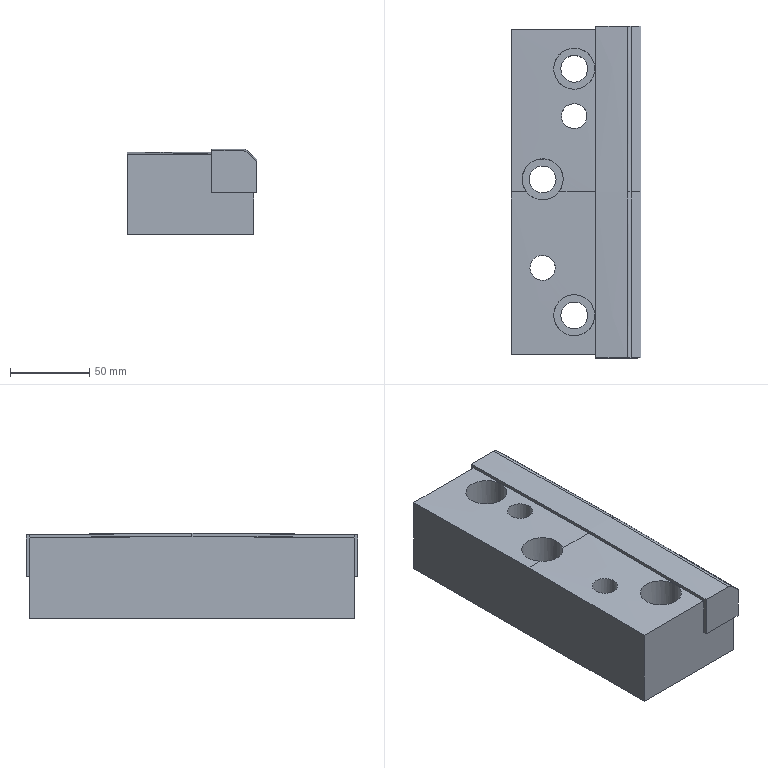Part | NX | features MAIN_BODY 2 | 1 solid | 43 faces | box 82.219 x 210 x 54.137 mm | volume 771248 mm3 | plane 18 | spline 16 | cylinder 9 | commonest cylinder face diameters 17 x3 26 x3 16 x2 20 x1